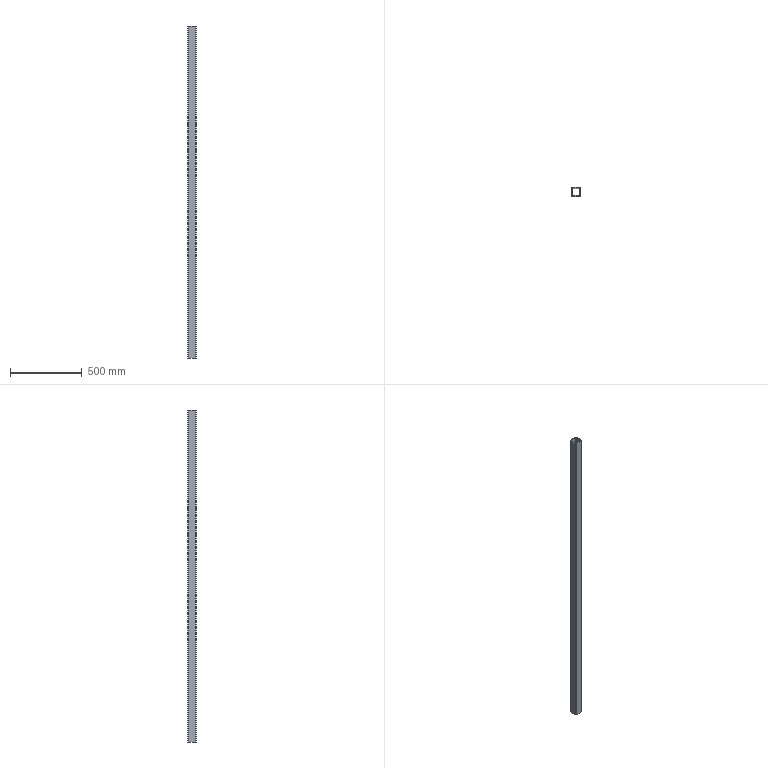Part | STEP file | 750038160 | 1 solid | 18 faces | box 60 x 60 x 2312 mm | volume 2008044 mm3 | plane 10 | cylinder 8 | commonest cylinder face diameters 4 x4 12 x4
STEP:
#1=CARTESIAN_POINT('',(-26.,24.,1156.));
#2=VERTEX_POINT('',#1);
#3=CARTESIAN_POINT('',(-26.,24.,-1156.));
#4=VERTEX_POINT('',#3);
#5=CARTESIAN_POINT('',(-26.,24.,1156.));
#6=DIRECTION('',(0.,0.,-1.));
#7=VECTOR('',#6,1000.);
#8=LINE('',#5,#7);
#9=EDGE_CURVE('',#2,#4,#8,.T.);
#10=ORIENTED_EDGE('',*,*,#9,.F.);
#11=CARTESIAN_POINT('',(-26.,-24.,1156.));
#12=VERTEX_POINT('',#11);
#13=CARTESIAN_POINT('',(-26.,-24.,1156.));
#14=DIRECTION('',(0.,1.,0.));
#15=VECTOR('',#14,1000.);
#16=LINE('',#13,#15);
#17=EDGE_CURVE('',#12,#2,#16,.T.);
#18=ORIENTED_EDGE('',*,*,#17,.F.);
#19=CARTESIAN_POINT('',(-26.,-24.,-1156.));
#20=VERTEX_POINT('',#19);
#21=CARTESIAN_POINT('',(-26.,-24.,1156.));
#22=DIRECTION('',(0.,0.,1.));
#23=VECTOR('',#22,1000.);
#24=LINE('',#21,#23);
#25=EDGE_CURVE('',#20,#12,#24,.T.);
#26=ORIENTED_EDGE('',*,*,#25,.F.);
#27=CARTESIAN_POINT('',(-26.,-24.,-1156.));
#28=DIRECTION('',(0.,-1.,0.));
#29=VECTOR('',#28,1000.);
#30=LINE('',#27,#29);
#31=EDGE_CURVE('',#4,#20,#30,.T.);
#32=ORIENTED_EDGE('',*,*,#31,.F.);
#33=EDGE_LOOP('',(#10,#18,#26,#32));
#34=FACE_OUTER_BOUND('',#33,.T.);
#35=CARTESIAN_POINT('',(-26.,-24.,1156.));
#36=DIRECTION('',(-1.,0.,0.));
#37=DIRECTION('',(0.,-1.,0.));
#38=AXIS2_PLACEMENT_3D('',#35,#36,#37);
#39=PLANE('',#38);
#40=ADVANCED_FACE('',(#34),#39,.F.);
#41=CARTESIAN_POINT('',(26.,24.,-1156.));
#42=VERTEX_POINT('',#41);
#43=CARTESIAN_POINT('',(24.,26.,-1156.));
#44=VERTEX_POINT('',#43);
#45=CARTESIAN_POINT('',(24.,24.,-1156.));
#46=DIRECTION('',(0.,0.,1.));
#47=DIRECTION('',(-1.,0.,0.));
#48=AXIS2_PLACEMENT_3D('',#45,#46,#47);
#49=CIRCLE('',#48,2.);
#50=EDGE_CURVE('',#42,#44,#49,.T.);
#51=ORIENTED_EDGE('',*,*,#50,.T.);
#52=CARTESIAN_POINT('',(-24.,26.,-1156.));
#53=VERTEX_POINT('',#52);
#54=CARTESIAN_POINT('',(24.,26.,-1156.));
#55=DIRECTION('',(-1.,0.,0.));
#56=VECTOR('',#55,1000.);
#57=LINE('',#54,#56);
#58=EDGE_CURVE('',#44,#53,#57,.T.);
#59=ORIENTED_EDGE('',*,*,#58,.T.);
#60=CARTESIAN_POINT('',(-24.,24.,-1156.));
#61=DIRECTION('',(0.,0.,1.));
#62=DIRECTION('',(-1.,0.,0.));
#63=AXIS2_PLACEMENT_3D('',#60,#61,#62);
#64=CIRCLE('',#63,2.);
#65=EDGE_CURVE('',#53,#4,#64,.T.);
#66=ORIENTED_EDGE('',*,*,#65,.T.);
#67=ORIENTED_EDGE('',*,*,#31,.T.);
#68=CARTESIAN_POINT('',(-24.,-26.,-1156.));
#69=VERTEX_POINT('',#68);
#70=CARTESIAN_POINT('',(-24.,-24.,-1156.));
#71=DIRECTION('',(0.,0.,1.));
#72=DIRECTION('',(-1.,0.,0.));
#73=AXIS2_PLACEMENT_3D('',#70,#71,#72);
#74=CIRCLE('',#73,2.);
#75=EDGE_CURVE('',#20,#69,#74,.T.);
#76=ORIENTED_EDGE('',*,*,#75,.T.);
#77=CARTESIAN_POINT('',(24.,-26.,-1156.));
#78=VERTEX_POINT('',#77);
#79=CARTESIAN_POINT('',(24.,-26.,-1156.));
#80=DIRECTION('',(1.,0.,0.));
#81=VECTOR('',#80,1000.);
#82=LINE('',#79,#81);
#83=EDGE_CURVE('',#69,#78,#82,.T.);
#84=ORIENTED_EDGE('',*,*,#83,.T.);
#85=CARTESIAN_POINT('',(26.,-24.,-1156.));
#86=VERTEX_POINT('',#85);
#87=CARTESIAN_POINT('',(24.,-24.,-1156.));
#88=DIRECTION('',(0.,0.,1.));
#89=DIRECTION('',(-1.,0.,0.));
#90=AXIS2_PLACEMENT_3D('',#87,#88,#89);
#91=CIRCLE('',#90,2.);
#92=EDGE_CURVE('',#78,#86,#91,.T.);
#93=ORIENTED_EDGE('',*,*,#92,.T.);
#94=CARTESIAN_POINT('',(26.,-24.,-1156.));
#95=DIRECTION('',(0.,1.,0.));
#96=VECTOR('',#95,1000.);
#97=LINE('',#94,#96);
#98=EDGE_CURVE('',#86,#42,#97,.T.);
#99=ORIENTED_EDGE('',*,*,#98,.T.);
#100=EDGE_LOOP('',(#51,#59,#66,#67,#76,#84,#93,#99));
#101=FACE_BOUND('',#100,.T.);
#102=CARTESIAN_POINT('',(-24.,30.,-1156.));
#103=VERTEX_POINT('',#102);
#104=CARTESIAN_POINT('',(24.,30.,-1156.));
#105=VERTEX_POINT('',#104);
#106=CARTESIAN_POINT('',(24.,30.,-1156.));
#107=DIRECTION('',(1.,0.,0.));
#108=VECTOR('',#107,1000.);
#109=LINE('',#106,#108);
#110=EDGE_CURVE('',#103,#105,#109,.T.);
#111=ORIENTED_EDGE('',*,*,#110,.T.);
#112=CARTESIAN_POINT('',(30.,24.,-1156.));
#113=VERTEX_POINT('',#112);
#114=CARTESIAN_POINT('',(24.,24.,-1156.));
#115=DIRECTION('',(0.,0.,-1.));
#116=DIRECTION('',(-1.,0.,0.));
#117=AXIS2_PLACEMENT_3D('',#114,#115,#116);
#118=CIRCLE('',#117,6.);
#119=EDGE_CURVE('',#105,#113,#118,.T.);
#120=ORIENTED_EDGE('',*,*,#119,.T.);
#121=CARTESIAN_POINT('',(30.,-24.,-1156.));
#122=VERTEX_POINT('',#121);
#123=CARTESIAN_POINT('',(30.,-24.,-1156.));
#124=DIRECTION('',(0.,-1.,0.));
#125=VECTOR('',#124,1000.);
#126=LINE('',#123,#125);
#127=EDGE_CURVE('',#113,#122,#126,.T.);
#128=ORIENTED_EDGE('',*,*,#127,.T.);
#129=CARTESIAN_POINT('',(24.,-30.,-1156.));
#130=VERTEX_POINT('',#129);
#131=CARTESIAN_POINT('',(24.,-24.,-1156.));
#132=DIRECTION('',(0.,0.,-1.));
#133=DIRECTION('',(-1.,0.,0.));
#134=AXIS2_PLACEMENT_3D('',#131,#132,#133);
#135=CIRCLE('',#134,6.);
#136=EDGE_CURVE('',#122,#130,#135,.T.);
#137=ORIENTED_EDGE('',*,*,#136,.T.);
#138=CARTESIAN_POINT('',(-24.,-30.,-1156.));
#139=VERTEX_POINT('',#138);
#140=CARTESIAN_POINT('',(24.,-30.,-1156.));
#141=DIRECTION('',(-1.,0.,0.));
#142=VECTOR('',#141,1000.);
#143=LINE('',#140,#142);
#144=EDGE_CURVE('',#130,#139,#143,.T.);
#145=ORIENTED_EDGE('',*,*,#144,.T.);
#146=CARTESIAN_POINT('',(-30.,-24.,-1156.));
#147=VERTEX_POINT('',#146);
#148=CARTESIAN_POINT('',(-24.,-24.,-1156.));
#149=DIRECTION('',(0.,0.,-1.));
#150=DIRECTION('',(-1.,0.,0.));
#151=AXIS2_PLACEMENT_3D('',#148,#149,#150);
#152=CIRCLE('',#151,6.);
#153=EDGE_CURVE('',#139,#147,#152,.T.);
#154=ORIENTED_EDGE('',*,*,#153,.T.);
#155=CARTESIAN_POINT('',(-30.,24.,-1156.));
#156=VERTEX_POINT('',#155);
#157=CARTESIAN_POINT('',(-30.,-24.,-1156.));
#158=DIRECTION('',(0.,1.,0.));
#159=VECTOR('',#158,1000.);
#160=LINE('',#157,#159);
#161=EDGE_CURVE('',#147,#156,#160,.T.);
#162=ORIENTED_EDGE('',*,*,#161,.T.);
#163=CARTESIAN_POINT('',(-24.,24.,-1156.));
#164=DIRECTION('',(0.,0.,-1.));
#165=DIRECTION('',(-1.,0.,0.));
#166=AXIS2_PLACEMENT_3D('',#163,#164,#165);
#167=CIRCLE('',#166,6.);
#168=EDGE_CURVE('',#156,#103,#167,.T.);
#169=ORIENTED_EDGE('',*,*,#168,.T.);
#170=EDGE_LOOP('',(#111,#120,#128,#137,#145,#154,#162,#169));
#171=FACE_OUTER_BOUND('',#170,.T.);
#172=CARTESIAN_POINT('',(24.,-24.,-1156.));
#173=DIRECTION('',(0.,0.,-1.));
#174=DIRECTION('',(-1.,0.,0.));
#175=AXIS2_PLACEMENT_3D('',#172,#173,#174);
#176=PLANE('',#175);
#177=ADVANCED_FACE('',(#101,#171),#176,.T.);
#178=CARTESIAN_POINT('',(-24.,26.,1156.));
#179=VERTEX_POINT('',#178);
#180=CARTESIAN_POINT('',(-24.,26.,1156.));
#181=DIRECTION('',(0.,0.,-1.));
#182=VECTOR('',#181,1000.);
#183=LINE('',#180,#182);
#184=EDGE_CURVE('',#179,#53,#183,.T.);
#185=ORIENTED_EDGE('',*,*,#184,.F.);
#186=CARTESIAN_POINT('',(-24.,24.,1156.));
#187=DIRECTION('',(0.,0.,-1.));
#188=DIRECTION('',(-1.,0.,0.));
#189=AXIS2_PLACEMENT_3D('',#186,#187,#188);
#190=CIRCLE('',#189,2.);
#191=EDGE_CURVE('',#2,#179,#190,.T.);
#192=ORIENTED_EDGE('',*,*,#191,.F.);
#193=ORIENTED_EDGE('',*,*,#9,.T.);
#194=ORIENTED_EDGE('',*,*,#65,.F.);
#195=EDGE_LOOP('',(#185,#192,#193,#194));
#196=FACE_OUTER_BOUND('',#195,.T.);
#197=CARTESIAN_POINT('',(-24.,24.,1156.));
#198=DIRECTION('',(0.,0.,-1.));
#199=DIRECTION('',(-1.,0.,0.));
#200=AXIS2_PLACEMENT_3D('',#197,#198,#199);
#201=CYLINDRICAL_SURFACE('',#200,2.);
#202=ADVANCED_FACE('',(#196),#201,.F.);
#203=CARTESIAN_POINT('',(24.,26.,1156.));
#204=VERTEX_POINT('',#203);
#205=CARTESIAN_POINT('',(24.,26.,1156.));
#206=DIRECTION('',(-1.,0.,0.));
#207=VECTOR('',#206,1000.);
#208=LINE('',#205,#207);
#209=EDGE_CURVE('',#204,#179,#208,.T.);
#210=ORIENTED_EDGE('',*,*,#209,.F.);
#211=CARTESIAN_POINT('',(26.,24.,1156.));
#212=VERTEX_POINT('',#211);
#213=CARTESIAN_POINT('',(24.,24.,1156.));
#214=DIRECTION('',(0.,0.,1.));
#215=DIRECTION('',(-1.,0.,0.));
#216=AXIS2_PLACEMENT_3D('',#213,#214,#215);
#217=CIRCLE('',#216,2.);
#218=EDGE_CURVE('',#212,#204,#217,.T.);
#219=ORIENTED_EDGE('',*,*,#218,.F.);
#220=CARTESIAN_POINT('',(26.,-24.,1156.));
#221=VERTEX_POINT('',#220);
#222=CARTESIAN_POINT('',(26.,-24.,1156.));
#223=DIRECTION('',(0.,1.,0.));
#224=VECTOR('',#223,1000.);
#225=LINE('',#222,#224);
#226=EDGE_CURVE('',#221,#212,#225,.T.);
#227=ORIENTED_EDGE('',*,*,#226,.F.);
#228=CARTESIAN_POINT('',(24.,-26.,1156.));
#229=VERTEX_POINT('',#228);
#230=CARTESIAN_POINT('',(24.,-24.,1156.));
#231=DIRECTION('',(0.,0.,1.));
#232=DIRECTION('',(-1.,0.,0.));
#233=AXIS2_PLACEMENT_3D('',#230,#231,#232);
#234=CIRCLE('',#233,2.);
#235=EDGE_CURVE('',#229,#221,#234,.T.);
#236=ORIENTED_EDGE('',*,*,#235,.F.);
#237=CARTESIAN_POINT('',(-24.,-26.,1156.));
#238=VERTEX_POINT('',#237);
#239=CARTESIAN_POINT('',(24.,-26.,1156.));
#240=DIRECTION('',(1.,0.,0.));
#241=VECTOR('',#240,1000.);
#242=LINE('',#239,#241);
#243=EDGE_CURVE('',#238,#229,#242,.T.);
#244=ORIENTED_EDGE('',*,*,#243,.F.);
#245=CARTESIAN_POINT('',(-24.,-24.,1156.));
#246=DIRECTION('',(0.,0.,1.));
#247=DIRECTION('',(-1.,0.,0.));
#248=AXIS2_PLACEMENT_3D('',#245,#246,#247);
#249=CIRCLE('',#248,2.);
#250=EDGE_CURVE('',#12,#238,#249,.T.);
#251=ORIENTED_EDGE('',*,*,#250,.F.);
#252=ORIENTED_EDGE('',*,*,#17,.T.);
#253=ORIENTED_EDGE('',*,*,#191,.T.);
#254=EDGE_LOOP('',(#210,#219,#227,#236,#244,#251,#252,#253));
#255=FACE_BOUND('',#254,.T.);
#256=CARTESIAN_POINT('',(24.,30.,1156.));
#257=VERTEX_POINT('',#256);
#258=CARTESIAN_POINT('',(30.,24.,1156.));
#259=VERTEX_POINT('',#258);
#260=CARTESIAN_POINT('',(24.,24.,1156.));
#261=DIRECTION('',(0.,0.,-1.));
#262=DIRECTION('',(-1.,0.,0.));
#263=AXIS2_PLACEMENT_3D('',#260,#261,#262);
#264=CIRCLE('',#263,6.);
#265=EDGE_CURVE('',#257,#259,#264,.T.);
#266=ORIENTED_EDGE('',*,*,#265,.F.);
#267=CARTESIAN_POINT('',(-24.,30.,1156.));
#268=VERTEX_POINT('',#267);
#269=CARTESIAN_POINT('',(24.,30.,1156.));
#270=DIRECTION('',(1.,0.,0.));
#271=VECTOR('',#270,1000.);
#272=LINE('',#269,#271);
#273=EDGE_CURVE('',#268,#257,#272,.T.);
#274=ORIENTED_EDGE('',*,*,#273,.F.);
#275=CARTESIAN_POINT('',(-30.,24.,1156.));
#276=VERTEX_POINT('',#275);
#277=CARTESIAN_POINT('',(-24.,24.,1156.));
#278=DIRECTION('',(0.,0.,-1.));
#279=DIRECTION('',(-1.,0.,0.));
#280=AXIS2_PLACEMENT_3D('',#277,#278,#279);
#281=CIRCLE('',#280,6.);
#282=EDGE_CURVE('',#276,#268,#281,.T.);
#283=ORIENTED_EDGE('',*,*,#282,.F.);
#284=CARTESIAN_POINT('',(-30.,-24.,1156.));
#285=VERTEX_POINT('',#284);
#286=CARTESIAN_POINT('',(-30.,-24.,1156.));
#287=DIRECTION('',(0.,1.,0.));
#288=VECTOR('',#287,1000.);
#289=LINE('',#286,#288);
#290=EDGE_CURVE('',#285,#276,#289,.T.);
#291=ORIENTED_EDGE('',*,*,#290,.F.);
#292=CARTESIAN_POINT('',(-24.,-30.,1156.));
#293=VERTEX_POINT('',#292);
#294=CARTESIAN_POINT('',(-24.,-24.,1156.));
#295=DIRECTION('',(0.,0.,-1.));
#296=DIRECTION('',(-1.,0.,0.));
#297=AXIS2_PLACEMENT_3D('',#294,#295,#296);
#298=CIRCLE('',#297,6.);
#299=EDGE_CURVE('',#293,#285,#298,.T.);
#300=ORIENTED_EDGE('',*,*,#299,.F.);
#301=CARTESIAN_POINT('',(24.,-30.,1156.));
#302=VERTEX_POINT('',#301);
#303=CARTESIAN_POINT('',(24.,-30.,1156.));
#304=DIRECTION('',(-1.,0.,0.));
#305=VECTOR('',#304,1000.);
#306=LINE('',#303,#305);
#307=EDGE_CURVE('',#302,#293,#306,.T.);
#308=ORIENTED_EDGE('',*,*,#307,.F.);
#309=CARTESIAN_POINT('',(30.,-24.,1156.));
#310=VERTEX_POINT('',#309);
#311=CARTESIAN_POINT('',(24.,-24.,1156.));
#312=DIRECTION('',(0.,0.,-1.));
#313=DIRECTION('',(-1.,0.,0.));
#314=AXIS2_PLACEMENT_3D('',#311,#312,#313);
#315=CIRCLE('',#314,6.);
#316=EDGE_CURVE('',#310,#302,#315,.T.);
#317=ORIENTED_EDGE('',*,*,#316,.F.);
#318=CARTESIAN_POINT('',(30.,-24.,1156.));
#319=DIRECTION('',(0.,-1.,0.));
#320=VECTOR('',#319,1000.);
#321=LINE('',#318,#320);
#322=EDGE_CURVE('',#259,#310,#321,.T.);
#323=ORIENTED_EDGE('',*,*,#322,.F.);
#324=EDGE_LOOP('',(#266,#274,#283,#291,#300,#308,#317,#323));
#325=FACE_OUTER_BOUND('',#324,.T.);
#326=CARTESIAN_POINT('',(24.,-24.,1156.));
#327=DIRECTION('',(0.,0.,-1.));
#328=DIRECTION('',(-1.,0.,0.));
#329=AXIS2_PLACEMENT_3D('',#326,#327,#328);
#330=PLANE('',#329);
#331=ADVANCED_FACE('',(#255,#325),#330,.F.);
#332=ORIENTED_EDGE('',*,*,#25,.T.);
#333=ORIENTED_EDGE('',*,*,#250,.T.);
#334=CARTESIAN_POINT('',(-24.,-26.,1156.));
#335=DIRECTION('',(0.,0.,1.));
#336=VECTOR('',#335,1000.);
#337=LINE('',#334,#336);
#338=EDGE_CURVE('',#69,#238,#337,.T.);
#339=ORIENTED_EDGE('',*,*,#338,.F.);
#340=ORIENTED_EDGE('',*,*,#75,.F.);
#341=EDGE_LOOP('',(#332,#333,#339,#340));
#342=FACE_OUTER_BOUND('',#341,.T.);
#343=CARTESIAN_POINT('',(-24.,-24.,1156.));
#344=DIRECTION('',(0.,0.,-1.));
#345=DIRECTION('',(-1.,0.,0.));
#346=AXIS2_PLACEMENT_3D('',#343,#344,#345);
#347=CYLINDRICAL_SURFACE('',#346,2.);
#348=ADVANCED_FACE('',(#342),#347,.F.);
#349=CARTESIAN_POINT('',(24.,26.,1156.));
#350=DIRECTION('',(0.,0.,-1.));
#351=VECTOR('',#350,1000.);
#352=LINE('',#349,#351);
#353=EDGE_CURVE('',#204,#44,#352,.T.);
#354=ORIENTED_EDGE('',*,*,#353,.F.);
#355=ORIENTED_EDGE('',*,*,#209,.T.);
#356=ORIENTED_EDGE('',*,*,#184,.T.);
#357=ORIENTED_EDGE('',*,*,#58,.F.);
#358=EDGE_LOOP('',(#354,#355,#356,#357));
#359=FACE_OUTER_BOUND('',#358,.T.);
#360=CARTESIAN_POINT('',(-24.,26.,1156.));
#361=DIRECTION('',(0.,1.,0.));
#362=DIRECTION('',(0.,0.,1.));
#363=AXIS2_PLACEMENT_3D('',#360,#361,#362);
#364=PLANE('',#363);
#365=ADVANCED_FACE('',(#359),#364,.F.);
#366=CARTESIAN_POINT('',(26.,24.,1156.));
#367=DIRECTION('',(0.,0.,-1.));
#368=VECTOR('',#367,1000.);
#369=LINE('',#366,#368);
#370=EDGE_CURVE('',#212,#42,#369,.T.);
#371=ORIENTED_EDGE('',*,*,#370,.F.);
#372=ORIENTED_EDGE('',*,*,#218,.T.);
#373=ORIENTED_EDGE('',*,*,#353,.T.);
#374=ORIENTED_EDGE('',*,*,#50,.F.);
#375=EDGE_LOOP('',(#371,#372,#373,#374));
#376=FACE_OUTER_BOUND('',#375,.T.);
#377=CARTESIAN_POINT('',(24.,24.,1156.));
#378=DIRECTION('',(0.,0.,-1.));
#379=DIRECTION('',(-1.,0.,0.));
#380=AXIS2_PLACEMENT_3D('',#377,#378,#379);
#381=CYLINDRICAL_SURFACE('',#380,2.);
#382=ADVANCED_FACE('',(#376),#381,.F.);
#383=CARTESIAN_POINT('',(26.,-24.,1156.));
#384=DIRECTION('',(0.,0.,-1.));
#385=VECTOR('',#384,1000.);
#386=LINE('',#383,#385);
#387=EDGE_CURVE('',#221,#86,#386,.T.);
#388=ORIENTED_EDGE('',*,*,#387,.F.);
#389=ORIENTED_EDGE('',*,*,#226,.T.);
#390=ORIENTED_EDGE('',*,*,#370,.T.);
#391=ORIENTED_EDGE('',*,*,#98,.F.);
#392=EDGE_LOOP('',(#388,#389,#390,#391));
#393=FACE_OUTER_BOUND('',#392,.T.);
#394=CARTESIAN_POINT('',(26.,24.,1156.));
#395=DIRECTION('',(1.,0.,0.));
#396=DIRECTION('',(0.,0.,-1.));
#397=AXIS2_PLACEMENT_3D('',#394,#395,#396);
#398=PLANE('',#397);
#399=ADVANCED_FACE('',(#393),#398,.F.);
#400=CARTESIAN_POINT('',(24.,-26.,1156.));
#401=DIRECTION('',(0.,0.,-1.));
#402=VECTOR('',#401,1000.);
#403=LINE('',#400,#402);
#404=EDGE_CURVE('',#229,#78,#403,.T.);
#405=ORIENTED_EDGE('',*,*,#404,.F.);
#406=ORIENTED_EDGE('',*,*,#235,.T.);
#407=ORIENTED_EDGE('',*,*,#387,.T.);
#408=ORIENTED_EDGE('',*,*,#92,.F.);
#409=EDGE_LOOP('',(#405,#406,#407,#408));
#410=FACE_OUTER_BOUND('',#409,.T.);
#411=CARTESIAN_POINT('',(24.,-24.,1156.));
#412=DIRECTION('',(0.,0.,-1.));
#413=DIRECTION('',(-1.,0.,0.));
#414=AXIS2_PLACEMENT_3D('',#411,#412,#413);
#415=CYLINDRICAL_SURFACE('',#414,2.);
#416=ADVANCED_FACE('',(#410),#415,.F.);
#417=ORIENTED_EDGE('',*,*,#338,.T.);
#418=ORIENTED_EDGE('',*,*,#243,.T.);
#419=ORIENTED_EDGE('',*,*,#404,.T.);
#420=ORIENTED_EDGE('',*,*,#83,.F.);
#421=EDGE_LOOP('',(#417,#418,#419,#420));
#422=FACE_OUTER_BOUND('',#421,.T.);
#423=CARTESIAN_POINT('',(24.,-26.,1156.));
#424=DIRECTION('',(0.,-1.,0.));
#425=DIRECTION('',(0.,0.,-1.));
#426=AXIS2_PLACEMENT_3D('',#423,#424,#425);
#427=PLANE('',#426);
#428=ADVANCED_FACE('',(#422),#427,.F.);
#429=ORIENTED_EDGE('',*,*,#265,.T.);
#430=CARTESIAN_POINT('',(30.,24.,1156.));
#431=DIRECTION('',(0.,0.,-1.));
#432=VECTOR('',#431,1000.);
#433=LINE('',#430,#432);
#434=EDGE_CURVE('',#259,#113,#433,.T.);
#435=ORIENTED_EDGE('',*,*,#434,.T.);
#436=ORIENTED_EDGE('',*,*,#119,.F.);
#437=CARTESIAN_POINT('',(24.,30.,1156.));
#438=DIRECTION('',(0.,0.,1.));
#439=VECTOR('',#438,1000.);
#440=LINE('',#437,#439);
#441=EDGE_CURVE('',#105,#257,#440,.T.);
#442=ORIENTED_EDGE('',*,*,#441,.T.);
#443=EDGE_LOOP('',(#429,#435,#436,#442));
#444=FACE_OUTER_BOUND('',#443,.T.);
#445=CARTESIAN_POINT('',(24.,24.,1156.));
#446=DIRECTION('',(0.,0.,-1.));
#447=DIRECTION('',(-1.,0.,0.));
#448=AXIS2_PLACEMENT_3D('',#445,#446,#447);
#449=CYLINDRICAL_SURFACE('',#448,6.);
#450=ADVANCED_FACE('',(#444),#449,.T.);
#451=ORIENTED_EDGE('',*,*,#273,.T.);
#452=ORIENTED_EDGE('',*,*,#441,.F.);
#453=ORIENTED_EDGE('',*,*,#110,.F.);
#454=CARTESIAN_POINT('',(-24.,30.,1156.));
#455=DIRECTION('',(0.,0.,1.));
#456=VECTOR('',#455,1000.);
#457=LINE('',#454,#456);
#458=EDGE_CURVE('',#103,#268,#457,.T.);
#459=ORIENTED_EDGE('',*,*,#458,.T.);
#460=EDGE_LOOP('',(#451,#452,#453,#459));
#461=FACE_OUTER_BOUND('',#460,.T.);
#462=CARTESIAN_POINT('',(-24.,30.,1156.));
#463=DIRECTION('',(0.,1.,0.));
#464=DIRECTION('',(-1.,0.,0.));
#465=AXIS2_PLACEMENT_3D('',#462,#463,#464);
#466=PLANE('',#465);
#467=ADVANCED_FACE('',(#461),#466,.T.);
#468=ORIENTED_EDGE('',*,*,#282,.T.);
#469=ORIENTED_EDGE('',*,*,#458,.F.);
#470=ORIENTED_EDGE('',*,*,#168,.F.);
#471=CARTESIAN_POINT('',(-30.,24.,1156.));
#472=DIRECTION('',(0.,0.,1.));
#473=VECTOR('',#472,1000.);
#474=LINE('',#471,#473);
#475=EDGE_CURVE('',#156,#276,#474,.T.);
#476=ORIENTED_EDGE('',*,*,#475,.T.);
#477=EDGE_LOOP('',(#468,#469,#470,#476));
#478=FACE_OUTER_BOUND('',#477,.T.);
#479=CARTESIAN_POINT('',(-24.,24.,1156.));
#480=DIRECTION('',(0.,0.,-1.));
#481=DIRECTION('',(-1.,0.,0.));
#482=AXIS2_PLACEMENT_3D('',#479,#480,#481);
#483=CYLINDRICAL_SURFACE('',#482,6.);
#484=ADVANCED_FACE('',(#478),#483,.T.);
#485=ORIENTED_EDGE('',*,*,#290,.T.);
#486=ORIENTED_EDGE('',*,*,#475,.F.);
#487=ORIENTED_EDGE('',*,*,#161,.F.);
#488=CARTESIAN_POINT('',(-30.,-24.,1156.));
#489=DIRECTION('',(0.,0.,1.));
#490=VECTOR('',#489,1000.);
#491=LINE('',#488,#490);
#492=EDGE_CURVE('',#147,#285,#491,.T.);
#493=ORIENTED_EDGE('',*,*,#492,.T.);
#494=EDGE_LOOP('',(#485,#486,#487,#493));
#495=FACE_OUTER_BOUND('',#494,.T.);
#496=CARTESIAN_POINT('',(-30.,-24.,1156.));
#497=DIRECTION('',(-1.,0.,0.));
#498=DIRECTION('',(0.,-1.,0.));
#499=AXIS2_PLACEMENT_3D('',#496,#497,#498);
#500=PLANE('',#499);
#501=ADVANCED_FACE('',(#495),#500,.T.);
#502=ORIENTED_EDGE('',*,*,#299,.T.);
#503=ORIENTED_EDGE('',*,*,#492,.F.);
#504=ORIENTED_EDGE('',*,*,#153,.F.);
#505=CARTESIAN_POINT('',(-24.,-30.,1156.));
#506=DIRECTION('',(0.,0.,1.));
#507=VECTOR('',#506,1000.);
#508=LINE('',#505,#507);
#509=EDGE_CURVE('',#139,#293,#508,.T.);
#510=ORIENTED_EDGE('',*,*,#509,.T.);
#511=EDGE_LOOP('',(#502,#503,#504,#510));
#512=FACE_OUTER_BOUND('',#511,.T.);
#513=CARTESIAN_POINT('',(-24.,-24.,1156.));
#514=DIRECTION('',(0.,0.,-1.));
#515=DIRECTION('',(-1.,0.,0.));
#516=AXIS2_PLACEMENT_3D('',#513,#514,#515);
#517=CYLINDRICAL_SURFACE('',#516,6.);
#518=ADVANCED_FACE('',(#512),#517,.T.);
#519=ORIENTED_EDGE('',*,*,#307,.T.);
#520=ORIENTED_EDGE('',*,*,#509,.F.);
#521=ORIENTED_EDGE('',*,*,#144,.F.);
#522=CARTESIAN_POINT('',(24.,-30.,1156.));
#523=DIRECTION('',(0.,0.,1.));
#524=VECTOR('',#523,1000.);
#525=LINE('',#522,#524);
#526=EDGE_CURVE('',#130,#302,#525,.T.);
#527=ORIENTED_EDGE('',*,*,#526,.T.);
#528=EDGE_LOOP('',(#519,#520,#521,#527));
#529=FACE_OUTER_BOUND('',#528,.T.);
#530=CARTESIAN_POINT('',(24.,-30.,1156.));
#531=DIRECTION('',(0.,-1.,0.));
#532=DIRECTION('',(1.,0.,0.));
#533=AXIS2_PLACEMENT_3D('',#530,#531,#532);
#534=PLANE('',#533);
#535=ADVANCED_FACE('',(#529),#534,.T.);
#536=ORIENTED_EDGE('',*,*,#316,.T.);
#537=ORIENTED_EDGE('',*,*,#526,.F.);
#538=ORIENTED_EDGE('',*,*,#136,.F.);
#539=CARTESIAN_POINT('',(30.,-24.,1156.));
#540=DIRECTION('',(0.,0.,1.));
#541=VECTOR('',#540,1000.);
#542=LINE('',#539,#541);
#543=EDGE_CURVE('',#122,#310,#542,.T.);
#544=ORIENTED_EDGE('',*,*,#543,.T.);
#545=EDGE_LOOP('',(#536,#537,#538,#544));
#546=FACE_OUTER_BOUND('',#545,.T.);
#547=CARTESIAN_POINT('',(24.,-24.,1156.));
#548=DIRECTION('',(0.,0.,-1.));
#549=DIRECTION('',(-1.,0.,0.));
#550=AXIS2_PLACEMENT_3D('',#547,#548,#549);
#551=CYLINDRICAL_SURFACE('',#550,6.);
#552=ADVANCED_FACE('',(#546),#551,.T.);
#553=ORIENTED_EDGE('',*,*,#322,.T.);
#554=ORIENTED_EDGE('',*,*,#543,.F.);
#555=ORIENTED_EDGE('',*,*,#127,.F.);
#556=ORIENTED_EDGE('',*,*,#434,.F.);
#557=EDGE_LOOP('',(#553,#554,#555,#556));
#558=FACE_OUTER_BOUND('',#557,.T.);
#559=CARTESIAN_POINT('',(30.,24.,1156.));
#560=DIRECTION('',(1.,0.,0.));
#561=DIRECTION('',(0.,0.,-1.));
#562=AXIS2_PLACEMENT_3D('',#559,#560,#561);
#563=PLANE('',#562);
#564=ADVANCED_FACE('',(#558),#563,.T.);
#565=CLOSED_SHELL('',(#40,#177,#202,#331,#348,#365,#382,#399,#416,#428,#450,#467,#484,#501,#518,#535,#552,#564));
#566=MANIFOLD_SOLID_BREP('',#565);
#567=CARTESIAN_POINT('',(0.,0.,0.));
#568=DIRECTION('',(0.,0.,1.));
#569=DIRECTION('',(1.,0.,0.));
#570=AXIS2_PLACEMENT_3D('',#567,#568,#569);
#571=(LENGTH_UNIT()NAMED_UNIT(*)SI_UNIT(.MILLI.,.METRE.));
#572=UNCERTAINTY_MEASURE_WITH_UNIT(LENGTH_MEASURE(0.00001),#571,'','');
#573=(NAMED_UNIT(*)PLANE_ANGLE_UNIT()SI_UNIT($,.RADIAN.));
#574=(NAMED_UNIT(*)SI_UNIT($,.STERADIAN.)SOLID_ANGLE_UNIT());
#575=(GEOMETRIC_REPRESENTATION_CONTEXT(3)GLOBAL_UNCERTAINTY_ASSIGNED_CONTEXT((#572))GLOBAL_UNIT_ASSIGNED_CONTEXT((#571,#573,#574))REPRESENTATION_CONTEXT('',''));
#576=ADVANCED_BREP_SHAPE_REPRESENTATION('',(#566,#570),#575);